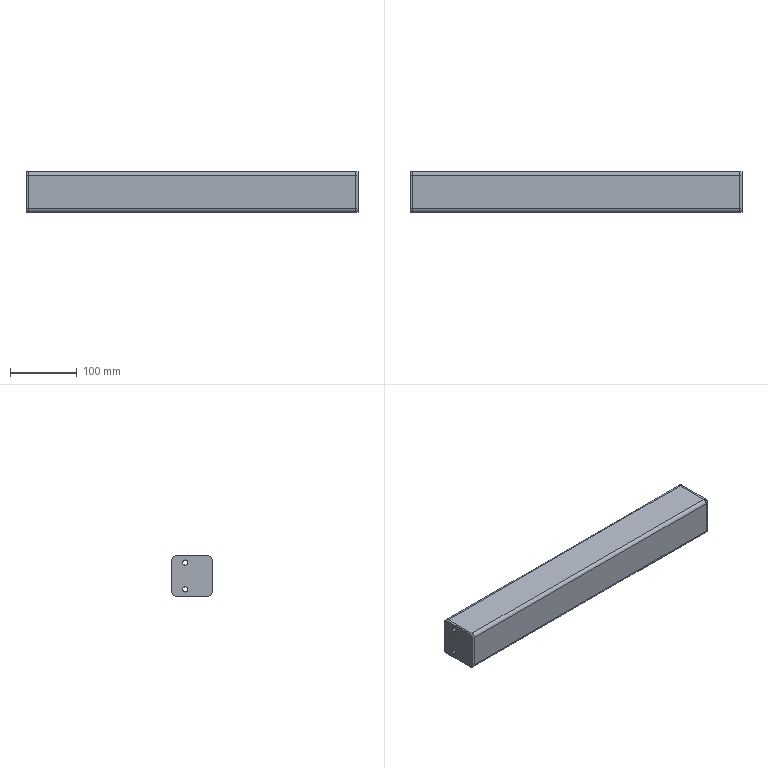Part | SolidWorks | features EdgeFlange 2, ICE 2, SMBaseFlange 2, FlatPattern 1, HoleWzd 1, LPattern 1, MirrorSolid 1, SheetMetal 1 | 3 solids | 66 faces | box 496 x 60 x 60 mm | volume 303095 mm3 | plane 42 | cylinder 24 | commonest cylinder face diameters 10 x12 8 x8 4 x4